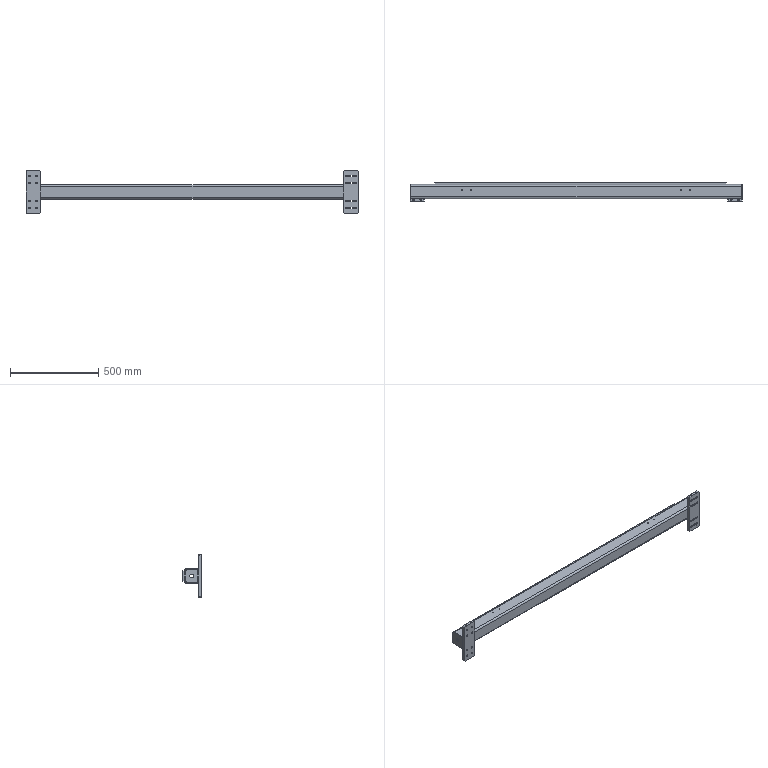Part | SolidWorks | features BaseBody 6 | 6 solids | 340 faces | box 1880 x 105 x 240 mm | volume 4723383 mm3 | cylinder 236 | plane 88 | cone 16 | commonest cylinder face diameters 6.8 x120 4.2 x24 5 x24 9 x24 15 x16 20 x16